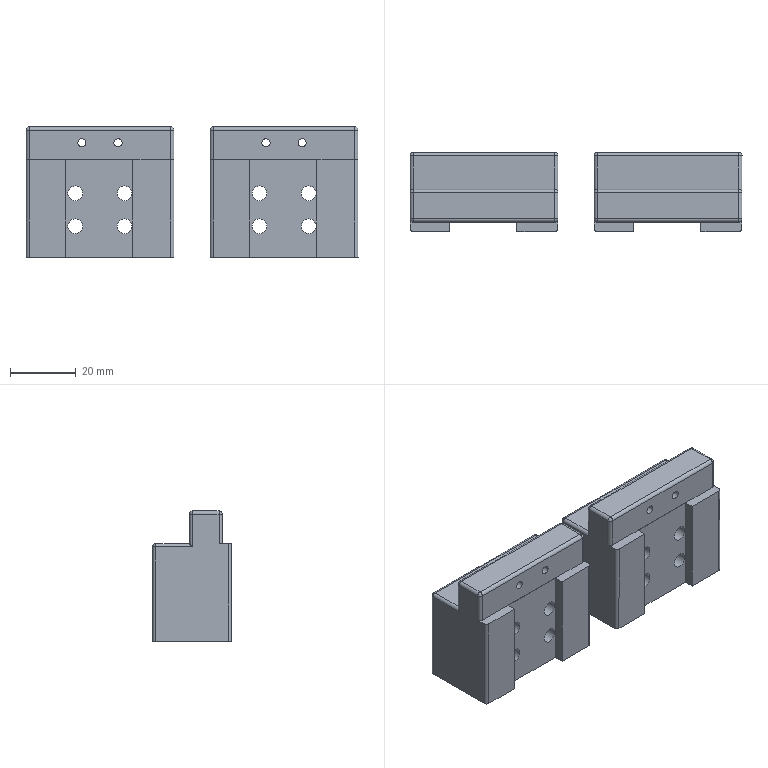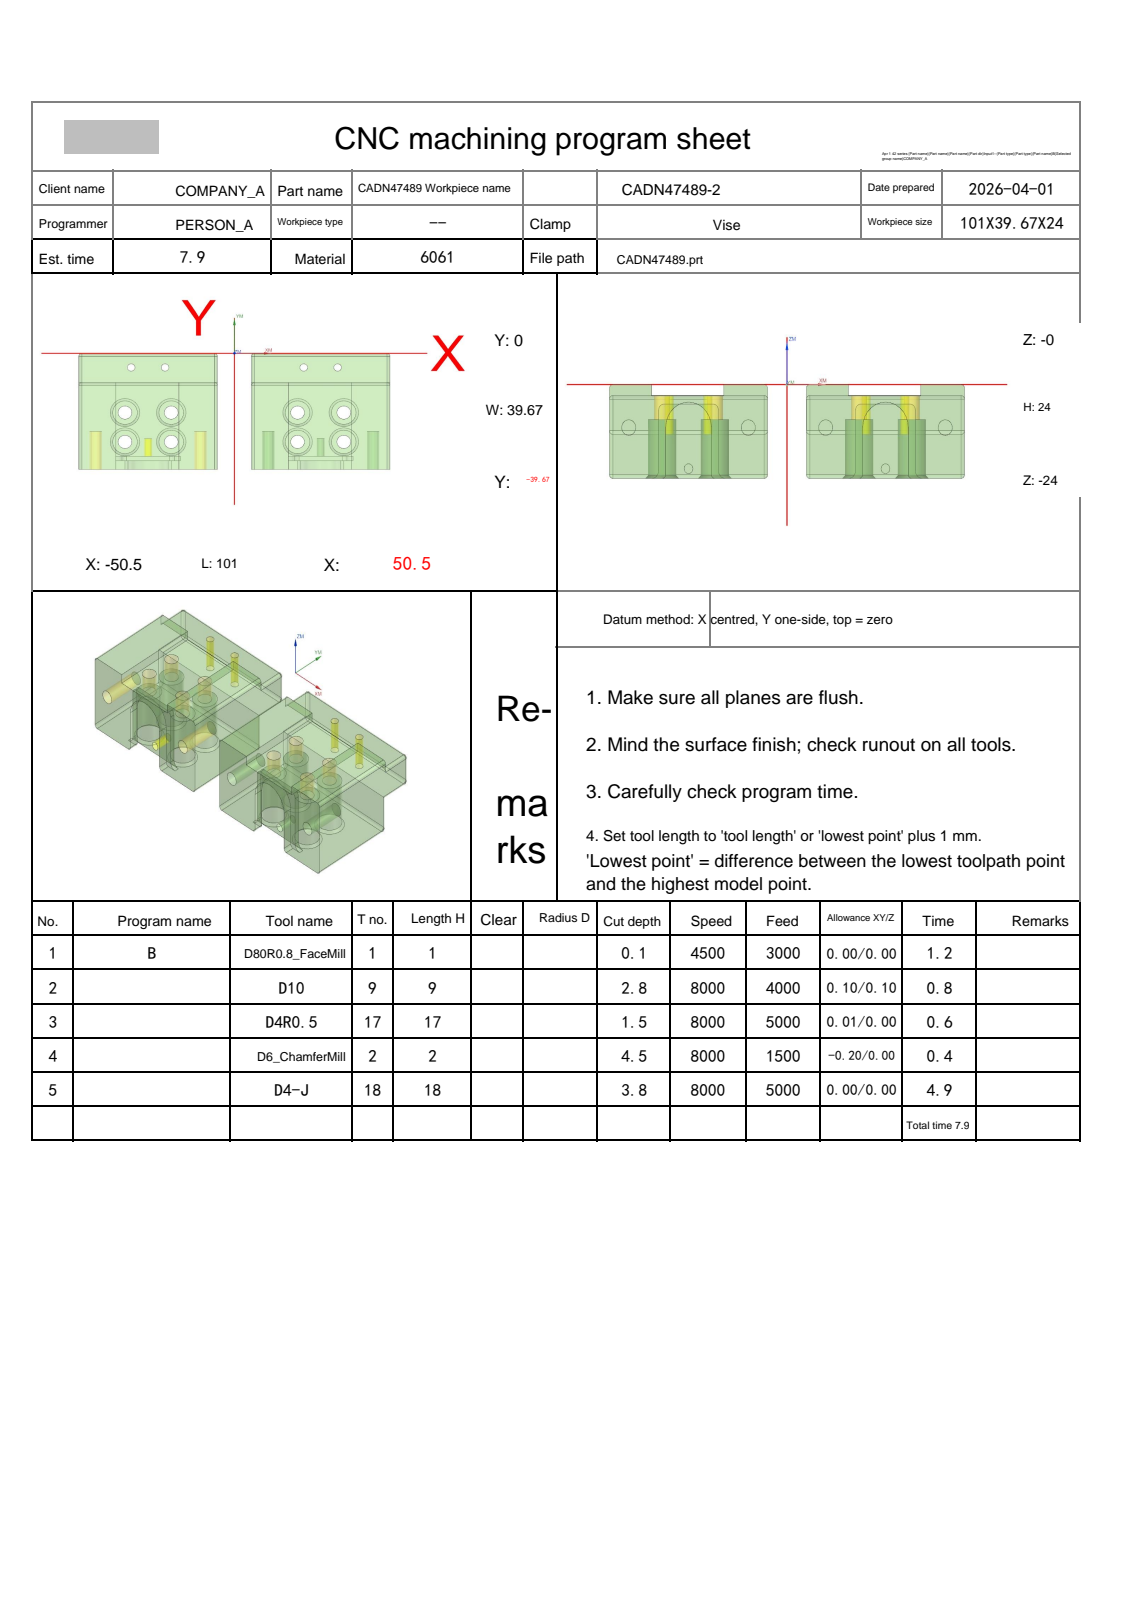NC program | NX | posted by the shop | part box 101.001 x 24.001 x 39.667 mm
Lines 1 to 1814 of 5289:
%
O0001
(Machine time: 8.72 MIN)
(===Total Tool:5===)
(T1=D80R0.8 face mill D=80.  R=0.8  D-  H01 Z=0.    )
(T9=D10     D=10.  R=0.   D-  H09 Z=-2.8  )
(T17=D4R0.5 D=4.   R=0.5  D-  H17 Z=-1.5  )
(T2=D6_ChamferMill   D=6.   R=0.   D-  H02 Z=-4.53 )
(T18=D4-J   D=4.   R=0.   D18 H18 Z=-3.78 )
G80 G90 G17 G49 G40
G91 G28 Z0
M01
N1 T01 M06
(D80R0.8 face mill  D=80. R=0.8 H=01 ce=0.20 di=0.10)
G00 G90 G54 X102.501 Y-19.833 M03 S4500
G43 H01 Z20.
M08
Z7.009
G01 Z5.009 F3000.
X90.501
X-90.5
X-102.5
Z7.009
G00 Z8.5
X102.501
Z6.518
G01 Z4.518
X90.501
X-90.5
X-102.5
Z6.518
G00 Z8.009
X102.501
Z6.027
G01 Z4.027
X90.501
X-90.5
X-102.5
Z6.027
G00 Z7.518
X102.501
Z5.536
G01 Z3.536
X90.501
X-90.5
X-102.5
Z5.536
G00 Z7.027
X102.501
Z5.045
G01 Z3.045
X90.501
X-90.5
X-102.5
Z5.045
G00 Z6.536
X102.501
Z4.555
G01 Z2.555
X90.501
X-90.5
X-102.5
Z4.555
G00 Z6.045
X102.501
Z4.064
G01 Z2.064
X90.501
X-90.5
X-102.5
Z4.064
G00 Z5.555
X102.501
Z3.573
G01 Z1.573
X90.501
X-90.5
X-102.5
Z3.573
G00 Z5.064
X102.501
Z3.082
G01 Z1.082
X90.501
X-90.5
X-102.5
Z3.082
G00 Z4.573
X102.501
Z2.591
G01 Z.591
X90.501
X-90.5
X-102.5
Z2.591
G00 Z4.082
X102.501
Z2.1
G01 Z.1
X90.501
X-90.5
X-102.5
Z2.1
G00 Z20.
G00 G90 X102.501 Y-19.833 M03 S4500
Z20.
Z2.
G01 Z0.0 F1000.
X90.501
X-90.5
X-102.5
Z2.
G00 Z20.
G91 G28 Z0.0
M05
M09
G91 G28 Z0.0
M01
N2 T09 M06
(D10  D=10. R=0. H=09 ce=0.10 di=0.10)
G00 G90 G54 X-35.251 Y12.178 M03 S8000
G43 H09 Z15.5
M08
Z.529
G01 Z-.671 F4000.
Y7.999
G03 X-28.251 Y.999 I7. J0.0
G01 X-6.421
X-6.42 Y-.925
X-6.409 Y-1.002
X-6.488 Y-1.003
X-6.528 Y-1.01
X-6.542 Y-1.035
X-6.553 Y-1.101
X-6.616 Y-1.077
X-7.12 Y-1.054
X-7.118 Y-3.501
Y-3.918
X-7.113 Y-4.817
X-5.519 Y-4.823
X-5.452 Y-4.819
X-5.462 Y-4.885
G03 X-5.74 Y-4.877 I-.278 J-5.432
X-6.175 Y-4.895 I0.0 J-5.439
G01 X-6.499 Y-4.901
X-16.07
X-18.
G03 X-18.883 Y-4.978 I0.0 J-5.1
X-20.293 Y-5.446 I.531 J-3.964
X-22.942 Y-8.743 I2.293 J-4.555
X-23.101 Y-9.921 I4.303 J-1.178
G01 X-23.1 Y-10.001
Y-35.568
X-23.099 Y-39.746
Y-39.758
X-23.1 Y-39.759
G03 X-19.738 Y-44.459 I5.104 J.097
X-19.133 Y-44.638 I1.742 J4.794
G01 X-19.136 Y-44.652
X-19.142 Y-44.724
X-19.212 Y-44.707
X-22.1
G02 X-24.422 Y-40.667 I4.105 J5.045
G01 X-32.078
G02 X-34.399 Y-44.708 I-6.424 J1.004
G01 X-37.235
X-37.296 Y-44.731
X-37.305 Y-44.667
X-37.315 Y-44.625
G03 X-33.401 Y-39.76 I-1.187 J4.962
G01 X-33.4 Y-39.759
Y-39.747
Y-35.569
Y-10.002
G03 X-33.757 Y-8.128 I-5.1 J0.0
X-34.123 Y-7.385 I-3.502 J-1.262
X-34.258 Y-7.171 I-4.377 J-2.617
X-34.942 Y-6.349 I-3.775 J-2.443
X-35.228 Y-6.09 I-3.559 J-3.653
X-36.405 Y-5.344 I-3.229 J-3.794
X-38.458 Y-4.902 I-2.053 J-4.54
G01 X-38.5
X-41.962
X-49.105
G03 X-49.816 Y-4.882 I-.711 J-12.782
X-50.517 Y-4.901 I0.0 J-12.802
G01 X-50.522 Y-4.816
X-50.437 Y-4.82
X-49.581
Y.998
X-29.441 Y.999
G02 X-28.495 Y.322 I0.0 J-1.
G01 X-27.388 Y-2.923
G03 X-26.752 Y-3.55 I.946 J.323
G02 X-26.061 Y-4.501 I-.31 J-.951
X-26.206 Y-5.018 I-1. J0.0
G03 X-27.294 Y-7.596 I8.205 J-4.983
X-27.6 Y-9.908 I8.654 J-2.321
G01 Y-35.568
G02 X-28.198 Y-36.167 I-.6 J.001
G01 X-28.301
G02 X-28.9 Y-35.568 I.001 J.6
G01 Y-10.002
G03 X-29.548 Y-6.536 I-9.6 J0.0
X-30.288 Y-5.03 I-7.711 J-2.855
G02 X-30.439 Y-4.501 I.849 J.529
X-29.441 Y-3.501 I1. J0.0
G01 X-28.941
G03 X-21.941 Y3.499 I0.0 J7.
G01 Y12.178
Z.529
G00 Z3.
G01 X-35.251 F6000.
G00 Z-.142
G01 Z-1.342 F4000.
Y7.999
G03 X-28.251 Y.999 I7. J0.0
G01 X-6.421
X-6.42 Y-.925
X-6.409 Y-1.002
X-6.488 Y-1.003
X-6.528 Y-1.01
X-6.542 Y-1.035
X-6.553 Y-1.101
X-6.616 Y-1.077
X-7.12 Y-1.054
X-7.117 Y-4.817
X-5.523 Y-4.822
X-5.456 Y-4.815
X-5.462 Y-4.882
G03 X-5.718 Y-4.877 I-.256 J-5.78
X-5.937 Y-4.881 I0.0 J-5.786
X-6.175 Y-4.895 I.197 J-5.435
G01 X-6.498 Y-4.901
X-10.713
X-11.606
X-18.
G03 X-18.883 Y-4.978 I0.0 J-5.1
X-20.293 Y-5.446 I.532 J-3.964
X-22.943 Y-8.743 I2.293 J-4.556
X-23.101 Y-9.921 I4.303 J-1.178
G01 X-23.1 Y-10.001
Y-39.462
X-23.099 Y-39.746
Y-39.758
X-23.1 Y-39.759
G03 X-19.133 Y-44.638 I5.102 J.095
G01 X-19.136 Y-44.652
X-19.141 Y-44.724
X-19.212 Y-44.707
X-22.101
G02 X-24.422 Y-40.667 I4.105 J5.044
G01 X-32.078
G02 X-34.398 Y-44.708 I-6.424 J1.003
G01 X-37.235
X-37.296 Y-44.731
X-37.305 Y-44.666
X-37.315 Y-44.626
G03 X-33.401 Y-39.76 I-1.187 J4.962
G01 X-33.4 Y-39.759
Y-39.747
Y-35.569
Y-10.002
G03 X-33.757 Y-8.128 I-5.1 J0.0
X-34.123 Y-7.385 I-3.502 J-1.263
X-34.259 Y-7.17 I-4.378 J-2.617
X-34.941 Y-6.349 I-3.775 J-2.444
X-35.229 Y-6.089 I-3.56 J-3.652
X-38.458 Y-4.902 I-3.228 J-3.796
G01 X-38.5
X-44.641
X-45.534
X-49.106
G03 X-49.816 Y-4.882 I-.711 J-12.782
X-50.2 Y-4.888 I0.0 J-12.802
X-50.455 Y-4.882 I-.256 J-5.139
G01 X-50.515
Y-4.881
X-50.511 Y-4.806
X-50.437 Y-4.82
X-49.581
Y.998
X-29.441 Y.999
G02 X-28.495 Y.322 I0.0 J-1.
G01 X-27.389 Y-2.922
G03 X-26.752 Y-3.55 I.946 J.323
G02 X-26.062 Y-4.501 I-.309 J-.951
X-26.206 Y-5.018 I-1. J0.0
G03 X-27.294 Y-7.597 I8.205 J-4.983
X-27.6 Y-9.908 I8.655 J-2.32
G01 Y-35.569
G02 X-28.198 Y-36.167 I-.6 J.002
G01 X-28.301
G02 X-28.9 Y-35.569 I.002 J.6
G01 Y-10.002
G03 X-29.548 Y-6.535 I-9.6 J0.0
X-30.288 Y-5.03 I-7.711 J-2.855
G02 X-30.439 Y-4.501 I.849 J.528
X-29.441 Y-3.501 I1. J0.0
G01 X-28.941
G03 X-21.941 Y3.499 I0.0 J7.
G01 X-21.942 Y12.178
Z-.142
G00 Z2.329
G01 X-35.251 F6000.
G00 Z-.813
G01 Z-2.013 F4000.
Y7.999
G03 X-28.251 Y.999 I7. J0.0
G01 X-6.421
X-6.42 Y-.925
X-6.409 Y-1.002
X-6.488 Y-1.003
X-6.528 Y-1.01
X-6.542 Y-1.035
X-6.553 Y-1.101
X-6.616 Y-1.077
X-7.12 Y-1.054
X-7.117 Y-4.817
X-5.54 Y-4.82
X-5.465 Y-4.807
X-5.462 Y-4.882
G03 X-5.718 Y-4.877 I-.256 J-5.78
X-5.937 Y-4.881 I0.0 J-5.786
X-6.175 Y-4.895 I.197 J-5.435
G01 X-6.497 Y-4.901
X-17.855
X-17.998 Y-4.899
G03 X-18.923 Y-4.984 I0.0 J-5.102
X-20.271 Y-5.433 I.572 J-3.958
X-22.943 Y-8.743 I2.273 J-4.568
X-23.101 Y-9.921 I4.303 J-1.178
G01 X-23.1 Y-10.001
X-23.099 Y-39.746
Y-39.758
X-23.1 Y-39.759
G03 X-19.133 Y-44.639 I5.101 J.094
G01 X-19.136 Y-44.651
X-19.141 Y-44.724
X-19.212 Y-44.707
X-22.102
G02 X-24.422 Y-40.667 I4.104 J5.043
G01 X-32.077
G02 X-34.397 Y-44.708 I-6.424 J1.002
G01 X-37.235
X-37.297 Y-44.731
X-37.306 Y-44.665
X-37.315 Y-44.627
G03 X-33.401 Y-39.76 I-1.186 J4.961
G01 X-33.4 Y-39.759
Y-39.747
Y-35.569
Y-10.002
G03 X-33.757 Y-8.128 I-5.1 J0.0
X-34.122 Y-7.385 I-3.502 J-1.263
X-34.259 Y-7.169 I-4.378 J-2.616
X-34.94 Y-6.35 I-3.774 J-2.444
X-35.231 Y-6.087 I-3.56 J-3.651
X-38.458 Y-4.902 I-3.226 J-3.797
G01 X-38.5
X-49.106
G03 X-49.816 Y-4.882 I-.71 J-12.782
X-50.199 Y-4.888 I0.0 J-12.802
X-50.456 Y-4.881 I-.257 J-5.138
G01 X-50.515 Y-4.882
X-50.51 Y-4.868
X-50.503 Y-4.8
X-50.437 Y-4.82
X-49.581
Y.998
X-29.442 Y.999
G02 X-28.495 Y.322 I0.0 J-1.
G01 X-27.389 Y-2.922
G03 X-26.752 Y-3.55 I.946 J.323
G02 X-26.062 Y-4.501 I-.309 J-.951
X-26.206 Y-5.018 I-1. J0.0
G03 X-27.265 Y-7.486 I8.208 J-4.984
X-27.6 Y-9.908 I8.625 J-2.427
G01 Y-35.569
G02 X-28.198 Y-36.167 I-.6 J.002
G01 X-28.302
G02 X-28.9 Y-35.569 I.002 J.6
G01 Y-10.002
G03 X-29.548 Y-6.535 I-9.6 J0.0
X-30.288 Y-5.029 I-7.711 J-2.856
G02 X-30.439 Y-4.501 I.849 J.528
X-29.441 Y-3.501 I1. J0.0
G01 X-28.941
G03 X-21.942 Y3.499 I0.0 J7.
G01 Y12.178
Z-.813
G00 Z1.658
G01 X-35.251 F6000.
G00 Z-1.484
G01 Z-2.684 F4000.
Y7.999
G03 X-28.251 Y.999 I7. J0.0
G01 X-6.421
X-6.42 Y-.925
X-6.409 Y-1.002
X-6.488 Y-1.003
X-6.528 Y-1.01
X-6.542 Y-1.035
X-6.553 Y-1.101
X-6.616 Y-1.077
X-7.12 Y-1.054
X-7.117 Y-4.817
X-5.539 Y-4.82
X-5.465 Y-4.807
X-5.462 Y-4.882
G03 X-5.718 Y-4.877 I-.256 J-5.78
X-5.937 Y-4.881 I0.0 J-5.786
X-6.175 Y-4.895 I.197 J-5.435
G01 X-6.496 Y-4.901
X-17.855
X-17.999 Y-4.899
G03 X-18.931 Y-4.985 I0.0 J-5.101
X-20.259 Y-5.427 I.579 J-3.957
X-22.947 Y-8.76 I2.26 J-4.573
X-23.101 Y-9.921 I4.308 J-1.161
G01 X-23.1 Y-10.001
Y-39.42
G03 X-23.105 Y-39.657 I5.104 J-.237
X-20.843 Y-43.9 I5.11 J0.0
X-19.133 Y-44.639 I2.845 J4.235
G01 X-19.136 Y-44.651
X-19.141 Y-44.724
X-19.212 Y-44.707
X-22.103
G02 X-24.426 Y-40.667 I4.107 J5.051
G01 X-32.073
G02 X-34.397 Y-44.708 I-6.432 J1.01
G01 X-37.235
X-37.297 Y-44.731
X-37.306 Y-44.665
X-37.315 Y-44.627
G03 X-35.543 Y-43.821 I-1.186 J4.961
X-33.394 Y-39.657 I-2.962 J4.165
X-33.4 Y-39.42 I-5.111 J0.0
G01 Y-35.569
Y-9.999
G03 X-33.453 Y-9.27 I-5.1 J-.002
X-33.758 Y-8.125 I-5.049 J-.732
X-33.898 Y-7.79 I-3.501 J-1.266
X-34.141 Y-7.354 I-3.367 J-1.592
X-34.268 Y-7.155 I-4.361 J-2.648
X-34.916 Y-6.373 I-3.765 J-2.459
X-35.284 Y-6.043 I-3.586 J-3.629
X-38.457 Y-4.902 I-3.173 J-3.842
G01 X-38.47
X-49.106
G03 X-49.816 Y-4.882 I-.71 J-12.782
X-50.199 Y-4.888 I0.0 J-12.802
X-50.456 Y-4.881 I-.257 J-5.138
G01 X-50.515 Y-4.882
X-50.512 Y-4.806
X-50.437 Y-4.82
X-49.581
Y.998
X-29.442 Y.999
G02 X-28.495 Y.322 I0.0 J-1.
G01 X-27.389 Y-2.923
G03 X-26.753 Y-3.55 I.946 J.323
G02 X-26.062 Y-4.501 I-.31 J-.951
X-26.206 Y-5.018 I-1. J0.0
G03 X-27.303 Y-7.631 I8.207 J-4.983
X-27.601 Y-9.92 I8.664 J-2.289
G01 X-27.6 Y-10.002
Y-35.569
G02 X-28.198 Y-36.167 I-.6 J.002
G01 X-28.302
G02 X-28.9 Y-35.569 I.002 J.6
G01 Y-9.997
G03 X-29. Y-8.624 I-9.6 J-.004
X-29.55 Y-6.53 I-9.502 J-1.377
X-29.835 Y-5.855 I-7.709 J-2.861
X-30.295 Y-5.018 I-7.425 J-3.533
G02 X-30.439 Y-4.501 I.856 J.517
X-29.442 Y-3.501 I1. J0.0
G01 X-28.942
G03 X-21.942 Y3.499 I0.0 J7.
G01 Y12.178
Z-1.484
G00 Z15.5
X-21.249 Y-51.707
Z-1.6
G01 Z-2.8
X-21.25 Y-47.667
G03 X-28.25 Y-40.667 I-7. J0.0
G01 X-32.073
G02 X-34.397 Y-44.708 I-6.432 J1.01
G01 X-37.235
X-37.297 Y-44.731
X-37.306 Y-44.665
X-37.315 Y-44.627
G03 X-36.984 Y-44.536 I-1.19 J4.97
X-35.865 Y-44.033 I-1.517 J4.87
X-33.394 Y-39.657 I-2.64 J4.376
X-33.4 Y-39.42 I-5.11 J0.0
G01 Y-15.101
X-23.1
Y-39.42
G03 X-23.105 Y-39.657 I5.104 J-.237
X-20.664 Y-44.014 I5.109 J0.0
X-19.133 Y-44.639 I2.666 J4.35
G01 X-19.136 Y-44.651
X-19.141 Y-44.724
X-19.212 Y-44.707
X-22.103
G02 X-24.426 Y-40.667 I4.107 J5.05
G01 X-28.198
G02 X-29.198 Y-39.667 I0.0 J1.
X-29.164 Y-39.41 I1. J0.0
G01 X-28.501 Y-36.917
G03 X-28.468 Y-36.66 I-.967 J.256
X-28.738 Y-35.977 I-1. J0.0
G02 X-28.9 Y-35.569 I.438 J.41
G01 Y-20.199
G02 X-28.302 Y-19.601 I.6 J-.002
G01 X-28.198
G02 X-27.6 Y-20.199 I-.002 J-.6
G01 Y-35.569
G02 X-28.198 Y-36.167 I-.6 J.002
G01 X-28.302
G02 X-28.669 Y-36.04 I.002 J.6
G03 X-30.823 Y-35.298 I-2.154 J-2.759
X-31.251 Y-35.325 I0.0 J-3.5
G01 X-31.25 Y-51.708
Z-1.6
G00 Z15.5
X-34.986 Y12.178
Z-1.6
G01 Z-2.8
G03 X-27.986 Y5.178 I7. J0.0
G01 X-8.202 Y5.179
X-6.501
X-6.416 Y5.183
X-6.421 Y5.099
Y4.469
X-49.58 Y4.468
X-49.552 Y5.102
X-49.555 Y5.185
X-49.472 Y5.178
X-27.986
X-27.486
G03 X-20.486 Y12.178 I0.0 J7.
G01 Z-1.6
G00 Z3.
G01 X20.749 Y12.179 F6000.
G00 Z.529
G01 Z-.671 F4000.
Y8.
G03 X27.749 Y1. I7. J0.0
G01 X49.582 Y1.001
X49.587 Y-4.819
X50.46
X50.541 Y-4.811
X50.539 Y-4.892
X50.347 Y-4.889
G03 X50.001 Y-4.9 I0.0 J-5.232
G01 X49.84
X49.508
X47.076
X44.644
X41.072
X38.
G03 X32.9 Y-10. I0.0 J-5.1
G01 Y-10.433
Y-39.665
Y-39.69
G03 X35.366 Y-44.035 I5.061 J0.0
X36.568 Y-44.555 I2.593 J4.34
X36.875 Y-44.632 I1.393 J4.865
G01 X36.874 Y-44.693
X36.816 Y-44.675
X36.608 Y-44.706
X33.892 Y-44.708
G02 X31.574 Y-40.666 I4.069 J5.019
G01 X23.921
G02 X21.578 Y-44.717 I-6.423 J1.012
G01 X18.755 Y-44.719
X18.723 Y-44.712
X18.654 Y-44.682
X18.61 Y-44.634
G03 X19.182 Y-44.471 I-1.113 J4.98
X20.186 Y-43.991 I-1.682 J4.812
X22.599 Y-39.763 I-2.688 J4.337
G01 Y-39.762
X22.6 Y-39.746
Y-35.567
Y-10.001
G03 X17.5 Y-4.901 I-5.1 J0.0
G01 X15.18
X11.609
X6.498
G03 X5.991 Y-4.885 I-.507 J-8.049
X5.46 Y-4.903 I0.0 J-8.065
G01 Y-4.9
X5.455 Y-4.816
X5.54 Y-4.82
X6.502
X6.482 Y-1.071
X6.419 Y-.176
Y1.
X26.559
G02 X27.505 Y.323 I0.0 J-1.
G01 X28.611 Y-2.921
G03 X29.248 Y-3.549 I.946 J.323
G02 X29.939 Y-4.5 I-.309 J-.951
X29.795 Y-5.017 I-1. J0.0
G03 X28.4 Y-10. I8.205 J-4.983
G01 Y-35.567
G02 X27.802 Y-36.166 I-.6 J.002
G01 X27.699
G02 X27.1 Y-35.567 I.001 J.6
G01 Y-10.001
G03 X25.705 Y-5.017 I-9.6 J0.0
G02 X25.561 Y-4.5 I.856 J.517
X26.559 Y-3.5 I1. J0.0
G01 X27.059
G03 X34.059 Y3.5 I0.0 J7.
G01 X34.058 Y12.179
Z.529
G00 Z3.
G01 X20.748 F6000.
G00 Z-.142
G01 Z-1.342 F4000.
Y8.
G03 X27.748 Y1. I7. J0.0
G01 X49.582 Y1.001
X49.587 Y-4.819
X50.46
X50.541 Y-4.811
X50.539 Y-4.892
X50.347 Y-4.889
G03 X50.009 Y-4.9 I0.0 J-5.232
G01 X49.507
X43.751
X42.858
X37.994
G03 X32.9 Y-9.994 I0.0 J-5.094
G01 Y-35.567
Y-39.665
Y-39.69
G03 X34.868 Y-43.695 I5.061 J0.0
X36.87 Y-44.64 I3.12 J4.019
G01 X36.816 Y-44.675
X36.608 Y-44.706
X33.892 Y-44.708
G02 X31.574 Y-40.666 I4.069 J5.019
G01 X23.921
G02 X21.579 Y-44.717 I-6.423 J1.011
G01 X18.755 Y-44.719
X18.723 Y-44.712
X18.654 Y-44.682
X18.61 Y-44.634
G03 X22.599 Y-39.763 I-1.112 J4.979
G01 Y-39.762
X22.6 Y-39.746
Y-37.684
Y-10.001
G03 X17.5 Y-4.901 I-5.1 J0.0
G01 X11.609
X6.497
G03 X5.991 Y-4.885 I-.506 J-8.049
X5.46 Y-4.903 I0.0 J-8.065
G01 X5.473 Y-4.856
X5.483 Y-4.795
X5.54 Y-4.82
X6.502
X6.495 Y-3.499
X6.482 Y-1.071
X6.419 Y-.176
Y1.
X26.558
G02 X27.505 Y.323 I0.0 J-1.
G01 X28.611 Y-2.922
G03 X29.247 Y-3.549 I.946 J.323
G02 X29.936 Y-4.5 I-.311 J-.951
X29.792 Y-5.017 I-1. J0.0
G03 X28.4 Y-9.994 I8.202 J-4.978
G01 Y-35.567
G02 X27.802 Y-36.166 I-.6 J.002
G01 X27.699
G02 X27.1 Y-35.567 I.002 J.6
G01 Y-10.001
G03 X25.705 Y-5.017 I-9.6 J0.0
G02 X25.561 Y-4.5 I.856 J.517
X26.558 Y-3.5 I1. J0.0
G01 X27.058
G03 X34.058 Y3.5 I0.0 J7.
G01 Y12.179
Z-.142
G00 Z2.329
G01 X20.748 F6000.
G00 Z-.813
G01 Z-2.013 F4000.
Y8.
G03 X27.748 Y1. I7. J0.0
G01 X49.582 Y1.001
X49.587 Y-4.819
X50.46
X50.541 Y-4.811
X50.539 Y-4.892
X50.347 Y-4.889
G03 X50.009 Y-4.9 I0.0 J-5.232
G01 X49.529
X37.992
G03 X32.9 Y-9.993 I0.0 J-5.093
G01 Y-35.567
Y-39.665
Y-39.69
G03 X34.692 Y-43.553 I5.061 J0.0
X36.87 Y-44.64 I3.296 J3.875
G01 X36.816 Y-44.675
X36.608 Y-44.706
X33.892 Y-44.708
X33.786 Y-44.62
G02 X31.574 Y-40.666 I4.175 J4.931
G01 X23.921
G02 X21.58 Y-44.717 I-6.422 J1.01
G01 X18.755 Y-44.719
X18.723 Y-44.712
X18.654 Y-44.682
X18.611 Y-44.635
G03 X22.599 Y-39.763 I-1.112 J4.979
G01 Y-39.762
X22.6 Y-39.746
Y-39.495
Y-35.568
Y-10.001
G03 X17.5 Y-4.901 I-5.1 J0.0
G01 X6.493
G03 X5.977 Y-4.884 I-.515 J-8.05
X5.46 Y-4.901 I0.0 J-8.067
G01 Y-4.892
X5.459 Y-4.811
X5.54 Y-4.82
X6.502
X6.482 Y-1.071
X6.419 Y-.176
Y1.
X26.558
G02 X27.505 Y.323 I0.0 J-1.
G01 X28.611 Y-2.922
G03 X29.246 Y-3.549 I.946 J.323
G02 X29.935 Y-4.5 I-.311 J-.95
X29.792 Y-5.016 I-1. J0.0
G03 X28.4 Y-9.993 I8.201 J-4.977
G01 Y-35.568
G02 X27.802 Y-36.166 I-.6 J.002
G01 X27.698
G02 X27.1 Y-35.568 I.002 J.6
G01 Y-10.001
G03 X25.705 Y-5.017 I-9.6 J0.0
G02 X25.561 Y-4.5 I.856 J.517
X26.558 Y-3.5 I1. J0.0
G01 X27.058
G03 X34.058 Y3.5 I0.0 J7.
G01 Y12.179
Z-.813
G00 Z1.658
G01 X20.747 F6000.
G00 Z-1.484
G01 Z-2.684 F4000.
X20.748 Y8.
G03 X27.748 Y1. I7. J0.0
G01 X49.582 Y1.001
X49.587 Y-4.819
X50.46
X50.534 Y-4.805
X50.538 Y-4.881
X50.457 Y-4.88
G03 X50.006 Y-4.9 I0.0 J-5.143
G01 X49.551
X37.991
G03 X32.9 Y-9.992 I0.0 J-5.091
G01 Y-39.42
G03 X32.894 Y-39.669 I5.09 J-.249
X33.372 Y-41.824 I5.096 J0.0
X34.46 Y-43.344 I4.589 J2.135
X35.334 Y-44.017 I3.53 J3.675
X36.87 Y-44.64 I2.654 J4.34
G01 X36.816 Y-44.675
X36.608 Y-44.706
X33.891 Y-44.708
G02 X33.492 Y-44.355 I4.098 J5.039
X32.104 Y-42.416 I4.469 J4.666
X31.571 Y-40.666 I5.886 J2.748
G01 X23.925
G02 X22.322 Y-44.016 I-6.431 J1.019
X21.58 Y-44.717 I-4.823 J4.36
G01 X18.755 Y-44.719
X18.723 Y-44.712
X18.654 Y-44.682
X18.611 Y-44.635
G03 X21.283 Y-43.077 I-1.112 J4.979
X22.605 Y-39.647 I-3.789 J3.43
X22.6 Y-39.42 I-5.111 J0.0
G01 Y-10.001
G03 X17.5 Y-4.901 I-5.1 J0.0
G01 X6.496
G03 X5.975 Y-4.884 I-.521 J-8.05
X5.46 Y-4.901 I0.0 J-8.067
G01 X5.455 Y-4.815
X5.54 Y-4.82
X6.502
X6.495 Y-3.499
X6.482 Y-1.071
X6.419 Y-.176
Y1.
X26.558
G02 X27.504 Y.323 I0.0 J-1.
G01 X28.611 Y-2.922
G03 X29.246 Y-3.549 I.946 J.323
G02 X29.935 Y-4.5 I-.311 J-.95
X29.791 Y-5.016 I-1. J0.0
G03 X28.4 Y-9.992 I8.2 J-4.976
G01 Y-35.568
G02 X27.802 Y-36.166 I-.6 J.002
G01 X27.698
G02 X27.1 Y-35.568 I.002 J.6
G01 Y-10.001
G03 X25.705 Y-5.017 I-9.6 J0.0
G02 X25.561 Y-4.5 I.856 J.517
X26.558 Y-3.5 I1. J0.0
G01 X27.058
G03 X34.058 Y3.5 I0.0 J7.
G01 Y12.179
Z-1.484
G00 Z.987
G01 X21.009 F6000.
G00 Z-1.6
G01 Z-2.8 F4000.
G03 X28.009 Y5.179 I7. J0.0
G01 X47.769
X48.215 Y5.18
X49.498 Y5.179
X49.583 Y5.184
X49.578 Y5.099
X49.579 Y4.47
X6.42
X6.439 Y5.102
X6.435 Y5.185
X6.519 Y5.179
X7.144
X28.009
X28.509
G03 X35.509 Y12.179 I0.0 J7.
G01 Z-1.6
G00 Z15.5
X34.751 Y-51.708
Z-1.6
G01 Z-2.8
X34.75 Y-47.666
G03 X27.75 Y-40.666 I-7. J0.0
G01 X23.925
G02 X22.223 Y-44.123 I-6.431 J1.019
X21.58 Y-44.717 I-4.724 J4.467
G01 X18.755 Y-44.719
X18.723 Y-44.712
X18.654 Y-44.682
X18.611 Y-44.635
G03 X21.205 Y-43.161 I-1.112 J4.979
X22.605 Y-39.647 I-3.711 J3.514
X22.6 Y-39.42 I-5.111 J0.0
G01 Y-15.103
Y-15.1
X32.9
Y-39.42
G03 X32.894 Y-39.669 I5.09 J-.249
X33.372 Y-41.824 I5.096 J0.0
X34.524 Y-43.404 I4.589 J2.134
X36.87 Y-44.641 I3.462 J3.726
G01 X36.816 Y-44.675
X36.608 Y-44.706
X33.891 Y-44.708
G02 X33.492 Y-44.355 I4.094 J5.03
X32.104 Y-42.416 I4.469 J4.666
X31.571 Y-40.666 I5.886 J2.748
G01 X27.802
G02 X26.802 Y-39.666 I0.0 J1.
X26.836 Y-39.409 I1. J0.0
G01 X27.499 Y-36.916
G03 X27.532 Y-36.659 I-.967 J.257
X27.262 Y-35.976 I-1. J0.0
G02 X27.1 Y-35.568 I.438 J.41
G01 Y-20.198
G02 X27.698 Y-19.6 I.6 J-.002
G01 X27.802
G02 X28.4 Y-20.198 I-.002 J-.6
G01 Y-35.568
G02 X27.802 Y-36.166 I-.6 J.002
G01 X27.698
G02 X27.331 Y-36.039 I.002 J.6
G03 X25.177 Y-35.297 I-2.154 J-2.759
X24.749 Y-35.323 I0.0 J-3.5
G01 X24.761 Y-51.715
Z-1.6
G00 Z15.5
G91 G28 Z0.0
M05
M09
G91 G28 Z0.0
M01
N3 T17 M06
(D4R0.5  D=4. R=0.5 H=17 ce=0.01 di=0.00)
G00 G90 G54 X51.344 Y-5.693 M03 S8000
G43 H17 Z15.5
M08
Z.454
G01 Z-.046 F5000.
X51.253 Y-8.935
X51.251 Y-9.052
G03 X51.354 Y-9.974 I4.184 J0.0
G01 X51.349 Y-39.64
X51.224 Y-40.77
X51.273 Y-40.769 Z-.066
X51.422 Y-39.679
X51.425 Y-9.974
X51.312 Y-9.126
X51.311 Y-8.925
X51.382 Y-8.909 Z-.079
X51.418 Y-8.901 Z-.092
G03 X51.5 Y-9.974 I8.094 J.079
G01 X51.498 Y-39.64
X51.385 Y-40.766
X51.439 Y-40.765 Z-.107
X51.475 Z-.122
X51.577 Y-39.64
X51.579 Y-9.974
G02 X51.492 Y-8.9 I7.178 J1.125
G01 X51.537 Z-.141
X51.575 Z-.159
G03 X51.67 Y-9.974 I6.771 J.059
G01 X51.668 Y-39.64
X51.564 Y-40.765
X51.617 Z-.181
X51.649 Z-.203
G02 X51.737 Y-39.64 I33.576 J-2.072
G01 X51.738 Y-9.974
X51.653 Y-8.9
X51.718 Z-.227
X51.752 Z-.252
Y-8.979
G03 X51.83 Y-9.974 I6.334 J0.0
G01 Y-39.64
G03 X51.752 Y-40.743 I7.76 J-1.103
G01 Y-40.765
X51.8 Z-.279
X51.828 Z-.307
Y-40.762
G02 X51.904 Y-39.64 I8.349 J0.0
G01 X51.905 Y-9.974
G02 X51.828 Y-8.969 I6.598 J1.005
G01 X51.829 Y-8.9
X51.879 Z-.337
X51.913 Z-.367
Y-8.934
G03 X51.983 Y-9.974 I7.724 J0.0
G01 Y-39.64
G03 X51.913 Y-40.765 I9.941 J-1.183
G01 X51.96 Z-.4
X52.001 Z-.433
G02 X52.062 Y-39.64 I10.943 J-.033
G01 Y-9.974
G02 X52.001 Y-8.954 I8.389 J1.02
G01 Y-8.9
X52.036 Z-.469
X52.073 Z-.504
X52.072 Y-9.001
G03 X52.125 Y-9.974 I8.958 J0.0
G01 Y-39.64
G03 X52.073 Y-40.728 I11.314 J-1.087
G01 Y-40.765
X52.103 Z-.542
X52.133 Z-.579
Y-40.742
G02 X52.183 Y-39.64 I12.114 J0.0
G01 Y-9.974
G02 X52.132 Y-8.992 I9.412 J.982
G01 X52.133 Y-8.9
X52.164 Z-.619
X52.192 Z-.659
Y-8.987
G03 X52.244 Y-9.974 I9.328 J0.0
G01 Y-39.64
G03 X52.193 Y-40.75 I11.941 J-1.11
G01 Y-40.765
X52.224 Z-.701
X52.256 Z-.743
G02 X52.301 Y-39.64 I14.065 J-.001
G01 X52.304 Y-10.009
X52.3 Y-9.939
X52.298 Y-9.904
X52.27 Y-9.499
G02 X52.253 Y-9.047 I6.329 J.452
G01 X52.255 Y-8.9
X52.282 Y-8.906 Z-.787
X52.298 Y-8.909 Z-.83
X52.297 Y-9.044
G03 X52.344 Y-9.904 I7.883 J0.0
G01 X52.346 Y-9.992
Y-39.552
G02 X52.305 Y-40.206 I-5.151 J0.0
G01 X52.298 Y-40.761
X52.321 Z-.875
X52.338 Z-.921
X52.345 Y-40.206
G03 X52.384 Y-39.523 I-5.938 J.683
G01 Y-9.992
X52.383 Y-9.939
G02 X52.337 Y-9.034 I8.873 J.905
G01 X52.338 Y-8.92
X52.36 Y-8.927 Z-.967
X52.379 Y-8.932 Z-1.014
Y-8.985
G03 X52.422 Y-9.992 I11.705 J0.0
G01 Y-39.64
G03 X52.379 Y-40.73 I13.665 J-1.09
G01 Y-40.761
X52.393 Z-1.061
X52.416 Z-1.109
X52.42 Y-40.206
G03 X52.455 Y-39.552 I-6.157 J.653
G01 X52.454 Y-9.956
G02 X52.414 Y-9.016 I11.093 J.94
G01 X52.415 Y-8.944
X52.433 Y-8.955 Z-1.206
G03 X52.474 Y-9.992 I13.807 J.029
G01 Y-39.64
G03 X52.434 Y-40.673 I13.423 J-1.033
G01 X52.435 Y-40.762
X52.44 Z-1.255
X52.451 Z-1.304
Y-40.646
G02 X52.488 Y-39.64 I13.701 J0.0
G01 Y-9.992
G02 X52.448 Y-8.967 I15.932 J1.128
G01 X52.46 Y-8.976 Z-1.402
G03 X52.5 Y-9.992 I24.524 J.466
G01 X52.499 Y-39.64
G03 X52.466 Y-40.659 I15.416 J-1.019
G01 Y-40.762
X52.475 Z-1.5
X52.474 Y-40.624
G02 X52.51 Y-39.64 I13.384 J0.0
G01 X52.509 Y-9.956
G02 X52.468 Y-8.989 I14.246 J1.098
G00 Z15.5
X-4.405 Y-5.846
Z.454
G01 Z-.046
X-4.762 Y-8.913
X-4.638 Y-9.975
X-4.641 Y-39.641
X-4.779 Y-40.77
X-4.733 Y-40.769 Z-.066
X-4.594 Y-39.641
X-4.591 Y-9.975
X-4.71 Y-8.91
X-4.62 Y-8.906 Z-.079
X-4.602 Y-8.905 Z-.092
X-4.499 Y-9.975
X-4.5 Y-39.641
X-4.63 Y-40.768
X-4.562 Y-40.767 Z-.107
X-4.525 Y-40.766 Z-.122
X-4.425 Y-39.641
X-4.423 Y-9.975
G02 X-4.506 Y-8.937 I6.477 J1.038
G01 Y-8.901
X-4.463 Z-.141
X-4.427 Z-.159
Y-8.929
G03 X-4.336 Y-9.975 I6.071 J0.0
G01 X-4.338 Y-39.641
X-4.441 Y-40.766
X-4.383 Z-.181
X-4.36 Z-.203
G02 X-4.255 Y-39.641 I9.203 J-.294
G01 X-4.254 Y-9.975
G02 X-4.352 Y-8.922 I5.572 J1.053
G01 Y-8.901
X-4.285 Z-.227
X-4.237 Z-.252
Y-8.908
G03 X-4.174 Y-9.975 I9.048 J0.0
G01 X-4.175 Y-39.641
G03 X-4.238 Y-40.766 I11.999 J-1.232
G01 X-4.2 Z-.279
X-4.166 Z-.307
G02 X-4.101 Y-39.641 I11.11 J-.078
G01 X-4.1 Y-9.975
G02 X-4.166 Y-8.927 I8.344 J1.048
G01 Y-8.901
X-4.121 Z-.337
X-4.087 Z-.367
Y-8.944
G03 X-4.019 Y-9.975 I7.806 J0.0
G01 X-4.02 Y-39.641
G03 X-4.087 Y-40.766 I10.187 J-1.178
G01 X-4.04 Z-.4
X-4.002 Z-.433
G02 X-3.943 Y-39.641 I17.813 J-.366
G01 Y-9.975
G02 X-4.002 Y-8.901 I10.888 J1.138
G01 X-3.964 Z-.469
X-3.931 Z-.504
Y-8.986
G03 X-3.881 Y-9.975 I9.891 J0.0
G01 X-3.882 Y-39.641
G03 X-3.93 Y-40.755 I12.697 J-1.114
G01 Y-40.766
X-3.897 Z-.542
X-3.869 Z-.579
X-3.87 Y-40.748
G02 X-3.817 Y-39.641 I11.803 J0.0
G01 Y-9.975
G02 X-3.87 Y-8.992 I9.113 J.983
G01 Y-8.901
X-3.836 Z-.619
X-3.806 Z-.659
X-3.807 Y-9.02
G03 X-3.76 Y-9.975 I9.693 J0.0
G01 Y-39.641
G03 X-3.806 Y-40.724 I12.691 J-1.083
G01 Y-40.766
X-3.774 Z-.701
X-3.746 Z-.743
X-3.747 Y-40.613
G02 X-3.7 Y-39.641 I10.047 J0.0
G01 Y-9.975
G02 X-3.747 Y-9.073 I8.495 J.902
G01 X-3.746 Y-8.901
X-3.723 Z-.787
X-3.701 Z-.83
Y-9.011
G03 X-3.657 Y-9.904 I9.031 J0.0
G01 X-3.655 Y-9.975
Y-39.641
X-3.681 Y-40.101
X-3.692 Y-40.206
X-3.702 Y-40.766
X-3.678 Y-40.763 Z-.875
X-3.66 Y-40.762 Z-.921
G02 X-3.617 Y-39.641 I15.621 J-.041
G01 Y-9.975
G02 X-3.66 Y-8.994 I11.059 J.981
G01 Y-8.908
X-3.622 Y-8.92 Z-1.014
X-3.623 Y-9.028
G03 X-3.58 Y-9.922 I9.387 J0.0
G01 X-3.578 Y-9.992
Y-39.641
G03 X-3.621 Y-40.762 I16.324 J-1.188
G01 X-3.606 Z-1.061
X-3.586 Z-1.109
Y-40.645
G02 X-3.544 Y-39.641 I11.767 J0.0
G01 Y-9.975
G02 X-3.587 Y-9.119 I8.349 J.856
G01 X-3.585 Y-8.933
X-3.568 Y-8.944 Z-1.206
X-3.569 Y-9.013
G03 X-3.53 Y-9.904 I10.179 J0.0
G01 X-3.527 Y-39.541
G02 X-3.551 Y-40.122 I-7.016 J0.0
G03 X-3.57 Y-40.59 I5.642 J-.468
G01 X-3.568 Y-40.762
X-3.56 Z-1.255
X-3.55 Z-1.304
Y-40.747
G02 X-3.514 Y-39.641 I17.114 J0.0
G01 Y-9.975
G02 X-3.554 Y-8.957 I17.474 J1.19
G01 X-3.54 Y-8.971 Z-1.402
X-3.541 Y-9.127
X-3.513 Y-9.833
X-3.501 Y-9.975
Y-39.551
G02 X-3.534 Y-40.206 I-6.359 J0.0
G01 X-3.533 Y-40.762
X-3.527 Z-1.5
X-3.525 Y-40.206
G03 X-3.49 Y-39.529 I-6.43 J.677
G01 X-3.491 Y-10.01
G02 X-3.534 Y-8.982 I22.711 J1.465
G00 Z15.5
X4.78 Y-44.032
Z.454
G01 Z-.046
X4.758 Y-40.771
X4.755 Y-40.334
X4.642 Y-39.641
X4.638 Y-9.975
X4.772 Y-8.916
X4.72 Y-8.912 Z-.056
X4.715 Z-.066
X4.59 Y-9.975
X4.594 Y-39.641
G02 X4.714 Y-40.769 I-21.427 J-2.853
G01 X4.623 Y-40.767 Z-.079
X4.605 Z-.092
G03 X4.501 Y-39.641 I-11.948 J-.54
G01 X4.498 Y-9.975
X4.613 Y-8.906
X4.558 Y-8.903 Z-.107
X4.522 Y-8.901 Z-.122
X4.422 Y-9.975
X4.425 Y-39.641
G02 X4.507 Y-40.766 I-8.664 J-1.197
G01 X4.465 Z-.141
X4.428 Z-.159
G03 X4.338 Y-39.641 I-8.073 J-.08
G01 X4.335 Y-9.975
G03 X4.438 Y-8.901 I-8.147 J1.319
G01 X4.381 Z-.181
X4.358 Z-.203
G02 X4.253 Y-9.975 I-6.595 J.105
G01 X4.256 Y-39.641
G02 X4.353 Y-40.766 I-7.428 J-1.213
G01 X4.287 Z-.227
X4.238 Z-.252
G03 X4.175 Y-39.641 I-12.028 J-.106
G01 X4.174 Y-9.975
G03 X4.237 Y-8.908 I-8.998 J1.067
G01 Y-8.901
X4.198 Z-.279
X4.165 Z-.307
Y-8.926
G02 X4.1 Y-9.975 I-8.422 J0.0
G01 X4.101 Y-39.641
G02 X4.167 Y-40.766 I-11.018 J-1.202
G01 X4.123 Z-.337
X4.088 Z-.367
G03 X4.02 Y-39.641 I-10.237 J-.052
G01 X4.018 Y-9.975
G03 X4.087 Y-8.943 I-7.747 J1.031
G01 Y-8.901
X4.039 Z-.4
X4.001 Z-.433
G02 X3.942 Y-9.975 I-11.027 J.066
G01 X3.943 Y-39.641
G02 X4.002 Y-40.766 I-17.534 J-1.483
G01 X3.965 Z-.469
X3.931 Z-.504
Y-40.755
G03 X3.882 Y-39.641 I-12.753 J0.0
G01 X3.881 Y-9.975
G03 X3.931 Y-8.986 I-9.834 J.988
G01 X3.93 Y-8.901
X3.897 Z-.542
X3.869 Z-.579
X3.87 Y-8.991
G02 X3.817 Y-9.975 I-9.192 J0.0
G01 X3.818 Y-39.641
G02 X3.87 Y-40.747 I-11.724 J-1.106
G01 Y-40.766
X3.837 Z-.619
X3.807 Z-.659
Y-40.724
G03 X3.761 Y-39.641 I-12.748 J0.0
G01 X3.759 Y-9.975
G03 X3.807 Y-9.02 I-9.638 J.955
G01 X3.806 Y-8.901
X3.775 Z-.701
X3.745 Z-.743
X3.747 Y-9.075
G02 X3.699 Y-9.975 I-8.496 J0.0
G01 X3.7 Y-39.641
G02 X3.747 Y-40.614 I-10.124 J-.973
G01 X3.746 Y-40.766
X3.724 Z-.787
X3.701 Z-.83
G03 X3.655 Y-39.641 I-19.585 J-.222
G01 Y-9.992
Y-9.94
G03 X3.699 Y-9.01 I-9.866 J.93
G01 Y-8.901
X3.675 Y-8.905 Z-.875
X3.655 Y-8.909 Z-.921
X3.656 Y-9.058
G02 X3.617 Y-9.94 I-9.937 J0.0
G01 X3.616 Y-9.992
X3.617 Y-39.641
G02 X3.66 Y-40.762 I-18.288 J-1.253
G01 X3.64 Z-.967
X3.621 Z-1.014
G03 X3.579 Y-39.641 I-27.204 J-.467
G01 X3.578 Y-9.975
G03 X3.614 Y-9.042 I-12.196 J.933
G01 X3.613 Y-8.921
X3.576 Y-8.933 Z-1.109
X3.578 Y-9.122
G02 X3.543 Y-9.975 I-10.622 J0.0
G01 X3.544 Y-39.641
G02 X3.584 Y-40.762 I-23.164 J-1.382
G01 X3.57 Z-1.158
X3.553 Z-1.206
X3.522 Y-39.641
X3.521 Y-9.975
G03 X3.548 Y-9.102 I-14.213 J.873
G01 X3.547 Y-8.946
X3.528 Y-8.959 Z-1.304
Y-9.097
G02 X3.504 Y-9.957 I-14.945 J0.0
G01 X3.508 Y-39.641
X3.532 Y-40.762
X3.523 Z-1.353
X3.518 Z-1.402
X3.498 Y-39.641
Y-9.975
G03 X3.514 Y-9.11 I-24.197 J.864
G01 X3.513 Y-8.971
X3.505 Y-8.984 Z-1.5
G02 X3.506 Y-9.209 I-19.744 J-.225
X3.49 Y-10.01 I-19.746 J0.0
G01 X3.491 Y-39.641
X3.511 Y-40.762
G00 Z15.5
X-51.189 Y-44.041
Z.454
G01 Z-.046
X-51.241 Y-40.771
X-51.242 Y-40.765
G03 X-51.347 Y-39.641 I-7.016 J-.089
G01 X-51.353 Y-9.975
X-51.229 Y-8.949
X-51.28 Y-8.94 Z-.056
X-51.294 Y-8.937 Z-.066
X-51.303 Y-9.128
X-51.42 Y-9.933
X-51.424 Y-9.975
X-51.42 Y-39.682
G02 X-51.294 Y-40.769 I-5.302 J-1.166
G01 X-51.376 Y-40.767 Z-.079
X-51.413 Z-.092
Y-40.669
G03 X-51.496 Y-39.641 I-6.358 J0.0
G01 X-51.499 Y-9.975
X-51.392 Y-8.91
X-51.441 Y-8.905 Z-.107
X-51.476 Y-8.902 Z-.122
X-51.578 Y-9.975
X-51.575 Y-39.641
G02 X-51.488 Y-40.767 I-9.882 J-1.329
G01 X-51.534 Z-.141
X-51.572 Z-.159
G03 X-51.666 Y-39.641 I-9.298 J-.215
G01 X-51.669 Y-9.975
G03 X-51.565 Y-8.902 I-8.463 J1.363
G01 X-51.619 Z-.181
X-51.65 Z-.203
G02 X-51.737 Y-9.975 I-17.008 J.85
G01 X-51.735 Y-39.641
G02 X-51.651 Y-40.767 I-24.895 J-2.438
G01 X-51.715 Z-.227
X-51.75 Z-.252
Y-40.744
G03 X-51.829 Y-39.641 I-7.787 J0.0
G01 X-51.831 Y-9.975
G03 X-51.751 Y-8.984 I-6.12 J.991
G01 Y-8.902
X-51.801 Z-.279
X-51.828 Z-.307
Y-8.971
G02 X-51.905 Y-9.975 I-6.625 J0.0
G01 X-51.903 Y-39.641
G02 X-51.827 Y-40.765 I-8.291 J-1.125
G01 Y-40.767
X-51.877 Z-.337
X-51.912 Z-.367
G03 X-51.982 Y-39.641 I-10.1 J-.064
G01 X-51.983 Y-9.975
G03 X-51.913 Y-8.935 I-7.657 J1.041
G01 Y-8.902
X-51.961 Z-.4
X-52.001 Z-.433
Y-8.95
G02 X-52.062 Y-9.975 I-8.569 J0.0
G01 X-52.061 Y-39.641
G02 X-52. Y-40.767 I-11.12 J-1.171
G01 X-52.034 Z-.469
X-52.072 Z-.504
Y-40.733
G03 X-52.124 Y-39.641 I-11.424 J0.0
G01 X-52.125 Y-9.975
G03 X-52.072 Y-9.002 I-8.87 J.973
G01 X-52.073 Y-8.902
X-52.103 Z-.542
X-52.133 Z-.579
X-52.132 Y-8.994
G02 X-52.183 Y-9.975 I-9.466 J0.0
G01 X-52.182 Y-39.641
G02 X-52.132 Y-40.748 I-12.176 J-1.107
G01 Y-40.767
X-52.163 Z-.619
X-52.192 Z-.659
Y-40.756
G03 X-52.243 Y-39.641 I-12.132 J0.0
G01 X-52.244 Y-9.975
G03 X-52.192 Y-8.988 I-9.315 J.987
G01 X-52.193 Y-8.902
X-52.225 Z-.701
X-52.256 Z-.743
X-52.255 Y-8.991
G02 X-52.301 Y-9.975 I-10.615 J0.0
G01 X-52.3 Y-39.641
G02 X-52.255 Y-40.76 I-13.893 J-1.12
G01 Y-40.767
X-52.282 Y-40.763 Z-.787
X-52.297 Y-40.762 Z-.83
X-52.306 Y-40.206
G02 X-52.345 Y-39.549 I5.538 J.657
G01 X-52.346 Y-9.975
X-52.327 Y-9.675
X-52.316 Y-9.622
G03 X-52.299 Y-9.081 I-8.348 J.541
G01 X-52.3 Y-8.912
X-52.325 Y-8.918 Z-.875
X-52.343 Y-8.923 Z-.921
X-52.342 Y-9.057
G02 X-52.384 Y-9.975 I-10.124 J0.0
G01 X-52.383 Y-39.641
G02 X-52.338 Y-40.762 I-21.164 J-1.427
G01 X-52.36 Z-.967
X-52.379 Z-1.014
G03 X-52.422 Y-39.641 I-24.402 J-.367
G01 Y-9.975
G03 X-52.386 Y-9.101 I-10.408 J.874
G01 X-52.387 Y-8.934
X-52.421 Y-8.945 Z-1.109
X-52.42 Y-9.053
G02 X-52.456 Y-9.975 I-11.972 J0.0
G01 X-52.455 Y-39.641
G02 X-52.413 Y-40.762 I-30.437 J-1.695
G01 X-52.43 Z-1.158
X-52.446 Z-1.206
G03 X-52.478 Y-39.641 I-33.38 J-.387
G01 X-52.479 Y-9.975
G03 X-52.451 Y-9.083 I-14.561 J.892
G01 X-52.452 Y-8.957
X-52.476 Y-8.969 Z-1.304
X-52.475 Y-9.14
G02 X-52.496 Y-9.975 I-16.726 J0.0
G01 X-52.495 Y-39.641
X-52.468 Y-40.762
X-52.477 Z-1.353
X-52.482 Z-1.402
X-52.503 Y-39.641
X-52.504 Y-9.975
G03 X-52.487 Y-9.141 I-20.555 J.835
G01 Y-8.981
X-52.492 Y-8.993 Z-1.5
Y-9.028
G02 X-52.51 Y-10.011 I-27.571 J0.0
G01 Y-39.641
G02 X-52.49 Y-40.655 I-26.438 J-1.014
G01 Y-40.762
G00 Z15.5
G91 G28 Z0.0
M05
M09
G91 G28 Z0.0
M01
N4 T02 M06
(D6_ChamferMill  D=6. R=0. H=02 ce=0.00 di=0.00)
G00 G90 G54 X33.5 Y-4.85 M03 S8000
G43 H02 Z20.
M08
G98 G81 X33.5 Y-4.85 Z-4.534 R.216 F1000.
X22.5
X-22.5 Y-4.851
X-33.5 Z-4.535 R.215
G80
G00 Z20.
G00 G90 X-6.114 Y-40.893 M03 S6500
Z20.
Z.131
G01 Z-1.199 F1500.
G03 X-6.4 Y-40.693 I-1.286 J-1.532
G01 X-6.445 Y-40.663
X-6.5 Y-40.666
X-18.
G02 X-19. Y-39.666 I0.0 J1.
G01 Y-10.002
G02 X-18. Y-9.001 I1. J0.0
G01 X-6.5
X-6.446 Y-9.004
X-6.4 Y-8.974
G03 X-6.115 Y-8.774 I-1. J1.732
G01 Z.132
G00 Z10.
X6.114
Z.132
G01 Z-1.199
G03 X6.4 Y-8.974 I1.286 J1.532
G01 X6.445 Y-9.004
X6.5 Y-9.001
X17.5
G02 X18.5 Y-10.001 I0.0 J-1.
G01 Y-39.665
G02 X17.5 Y-40.665 I-1. J0.0
G01 X6.5 Y-40.666
X6.446 Y-40.663
X6.4 Y-40.692
G03 X6.115 Y-40.892 I1. J-1.732
G01 Z.131
G00 Z10.
X49.886
Z.131
G01 Z-1.199
G03 X49.6 Y-40.692 I-1.286 J-1.532
G01 X49.555 Y-40.662
X49.5 Y-40.665
X38.
G02 X37. Y-39.665 I0.0 J1.
G01 Y-10.001
G02 X38. Y-9.001 I1. J0.0
G01 X49.5 Y-9.
X49.554 Y-9.003
X49.6 Y-8.974
G03 X49.885 Y-8.774 I-1. J1.732
G01 Z.132
G00 Z10.
X33.247 Y-5.011
Z-2.329
G01 Z-3.983
G03 X33.438 Y-5.096 I.583 J1.049
G01 X33.468 Y-5.112
X33.5 Y-5.1
G03 X33.75 Y-4.85 I0.0 J.25
G01 X33.71 Y-4.715
X33.619 Y-4.631
X33.5 Y-4.6
X33.375 Y-4.634
X33.283 Y-4.725
X33.25 Y-4.85
X33.283 Y-4.975
X33.375 Y-5.067
X33.5 Y-5.1
X33.526 Y-5.114
X33.552 Y-5.1
X33.638 Y-5.083
X33.715 Y-5.041
Z-2.338
G00 Z-.233
X22.247 Y-5.011
Z-2.329
G01 Z-3.983
G03 X22.438 Y-5.096 I.583 J1.049
G01 X22.468 Y-5.112
X22.5 Y-5.1
G03 X22.75 Y-4.85 I0.0 J.25
G01 X22.71 Y-4.715
X22.619 Y-4.631
X22.5 Y-4.6
X22.375 Y-4.634
X22.283 Y-4.725
X22.25 Y-4.85
X22.283 Y-4.975
X22.375 Y-5.067
X22.5 Y-5.1
X22.526 Y-5.114
X22.552 Y-5.1
X22.638 Y-5.084
X22.715 Y-5.041
Z-2.338
G00 Z10.
X-22.716 Y-5.042
Z-2.339
G01 Z-3.983
X-22.639 Y-5.084
X-22.552 Y-5.101
X-22.526 Y-5.115
X-22.5 Y-5.101
X-22.375 Y-5.068
X-22.284 Y-4.976
X-22.25 Y-4.851
X-22.284 Y-4.726
X-22.375 Y-4.635
X-22.5 Y-4.601
X-22.625 Y-4.635
X-22.717 Y-4.726
X-22.75 Y-4.851
X-22.717 Y-4.976
X-22.625 Y-5.068
X-22.5 Y-5.101
X-22.474 Y-5.115
X-22.448 Y-5.101
X-22.362 Y-5.084
X-22.285 Y-5.042
Z-2.339
G00 Z-.233
X-33.716
Z-2.339
G01 Z-3.983
X-33.639 Y-5.084
X-33.552 Y-5.101
X-33.526 Y-5.115
X-33.5 Y-5.101
X-33.375 Y-5.068
X-33.284 Y-4.976
X-33.25 Y-4.851
X-33.284 Y-4.726
X-33.375 Y-4.635
X-33.5 Y-4.601
X-33.625 Y-4.635
X-33.717 Y-4.726
X-33.75 Y-4.851
X-33.717 Y-4.976
X-33.625 Y-5.068
X-33.5 Y-5.101
X-33.474 Y-5.115
X-33.448 Y-5.101
X-33.362 Y-5.084
X-33.285 Y-5.042
Z-2.339
G00 Z10.
X-21.007 Y-40.734
Z-1.794
G01 Z-4.099
X-21.093 Y-40.674
X-21.123 Y-40.666
X-35.377
X-35.407 Y-40.674
X-35.492 Y-40.734
Z-1.794
G00 Z-.349
X-35.3 Y-31.452
Z-1.803
G01 Z-4.099
X-35.232 Y-31.47
X-35.212 Y-31.468
G03 X-34.25 Y-30.252 I-.288 J1.216
X-34.571 Y-29.415 I-1.25 J0.0
G01 X-34.765 Y-29.24
X-34.991 Y-29.11
X-35.209 Y-29.039
X-35.23 Y-29.038
X-35.296 Y-29.058
Z-1.806
G00 Z-.349
X-35.3 Y-21.452
Z-1.802
G01 Z-4.099
X-35.232 Y-21.47
X-35.212 Y-21.468
G03 X-34.25 Y-20.252 I-.288 J1.216
X-34.571 Y-19.415 I-1.25 J0.0
G01 X-34.765 Y-19.24
X-34.992 Y-19.11
X-35.209 Y-19.039
X-35.23 Y-19.038
X-35.296 Y-19.058
Z-1.806
G00 Z10.
X-21.196 Y-19.266
Z-1.798
G01 Z-4.099
X-21.265 Y-19.274
X-21.283 Y-19.284
X-21.429 Y-19.415
G03 X-21.75 Y-20.249 I.922 J-.834
X-21.273 Y-21.229 I1.244 J0.0
G01 X-21.263 Y-21.232
X-21.229 Y-21.231
Z-1.831
G00 Z-.349
X-21.196 Y-29.266
Z-1.798
G01 Z-4.099
X-21.265 Y-29.274
X-21.283 Y-29.284
X-21.429 Y-29.415
G03 X-21.75 Y-30.249 I.922 J-.834
X-21.273 Y-31.229 I1.244 J0.0
G01 X-21.263 Y-31.232
X-21.228 Y-31.231
Z-1.831
G00 Z10.
X34.993 Y-40.733
Z-1.794
G01 Z-4.099
X34.907 Y-40.673
X34.877 Y-40.665
X20.623
X20.593 Y-40.673
X20.508 Y-40.733
Z-1.794
G00 Z-.349
X20.7 Y-31.451
Z-1.802
G01 Z-4.099
X20.768 Y-31.469
X20.788 Y-31.467
G03 X21.75 Y-30.251 I-.288 J1.216
X21.429 Y-29.414 I-1.25 J0.0
G01 X21.235 Y-29.239
X21.009 Y-29.109
X20.791 Y-29.038
X20.77 Y-29.037
X20.704 Y-29.057
Z-1.806
G00 Z-.349
X20.7 Y-21.451
Z-1.802
G01 Z-4.099
X20.768 Y-21.469
X20.788 Y-21.467
G03 X21.75 Y-20.251 I-.288 J1.216
X21.429 Y-19.414 I-1.25 J0.0
G01 X21.235 Y-19.239
X21.008 Y-19.109
X20.791 Y-19.038
X20.77 Y-19.037
X20.704 Y-19.057
Z-1.805
G00 Z10.
X34.804 Y-19.265
Z-1.797
G01 Z-4.099
X34.735 Y-19.273
X34.717 Y-19.283
X34.571 Y-19.414
G03 X34.25 Y-20.248 I.922 J-.834
X34.727 Y-21.228 I1.244 J0.0
G01 X34.737 Y-21.231
X34.771 Y-21.23
Z-1.83
G00 Z-.349
X34.804 Y-29.265
Z-1.798
G01 Z-4.099
X34.735 Y-29.273
X34.717 Y-29.283
G03 X34.252 Y-30.178 I.751 J-.958
G01 X34.25 Y-30.253
G03 X34.727 Y-31.228 I1.234 J0.0
G01 X34.737 Y-31.231
X34.772 Y-31.23
Z-1.831
G00 Z20.
G00 G90 X-37.7 Y-31.423 M03 S7000
Z20.
Z2.499
G01 Y-39.544 Z-.457 F1500.
X-37.736 Y-39.743 Z-.531
X-37.811 Y-39.931 Z-.605
X-37.923 Y-40.1 Z-.678
X-38.066 Y-40.244 Z-.752
X-38.235 Y-40.355 Z-.826
X-38.423 Y-40.43 Z-.899
X-38.622 Y-40.466 Z-.973
X-38.7 Z-1.001
X-50.3 Y-40.467
X-50.442 Y-40.456
X-50.581 Y-40.426
X-50.715 Y-40.376
X-50.84 Y-40.308
X-50.955 Y-40.222
X-51.055 Y-40.121
X-51.141 Y-40.007
X-51.209 Y-39.882
X-51.259 Y-39.748
X-51.29 Y-39.609
X-51.3 Y-39.467
Y-10.202 Z-1.
X-51.29 Y-10.06
X-51.26 Y-9.92
X-51.21 Y-9.787
X-51.141 Y-9.661
X-51.056 Y-9.547
X-50.955 Y-9.446
X-50.841 Y-9.361
X-50.716 Y-9.292
X-50.582 Y-9.242
X-50.443 Y-9.212
X-50.3 Y-9.202
X-38.7
X-38.558 Y-9.212
X-38.419 Y-9.242
X-38.285 Y-9.292
X-38.16 Y-9.361
X-38.045 Y-9.446
X-37.944 Y-9.547
X-37.859 Y-9.661
X-37.791 Y-9.786
X-37.741 Y-9.92
X-37.71 Y-10.059
X-37.7 Y-10.202
Y-39.466 Z-1.001
X-37.71 Y-39.609
X-37.74 Y-39.748
X-37.79 Y-39.882
X-37.858 Y-40.007
X-37.944 Y-40.121
X-38.045 Y-40.222
X-38.159 Y-40.308
X-38.284 Y-40.376
X-38.418 Y-40.426
X-38.557 Y-40.456
X-38.7 Y-40.466
X-39.2
Z1.499
G00 Z20.
G91 G28 Z0.0
M05
M09
G91 G28 Z0.0
M01